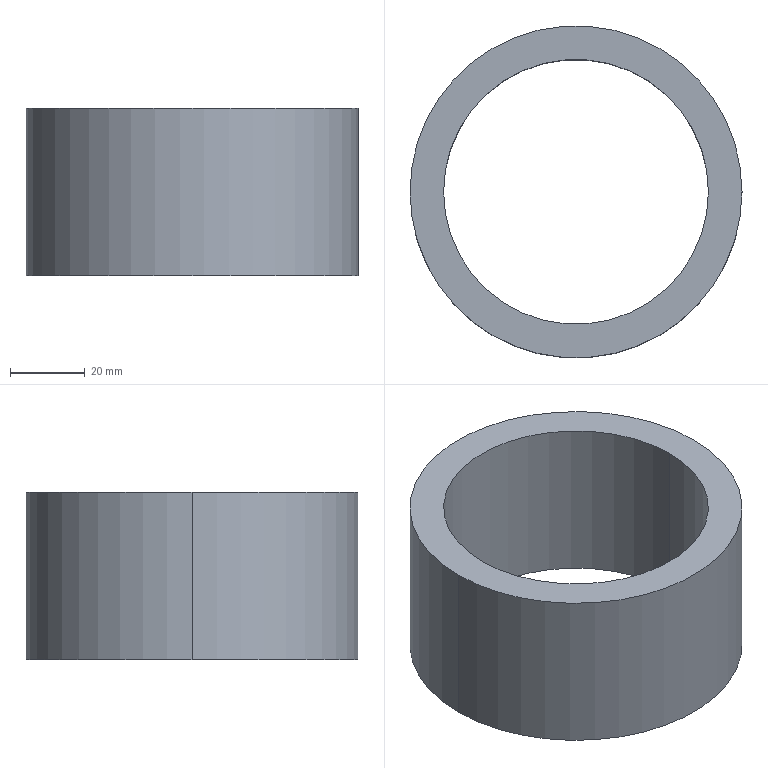Part | SolidWorks | features Extrusion 1 | 1 solid | 6 faces | box 89 x 89 x 45 mm | volume 101788 mm3 | cylinder 4 | plane 2 | commonest cylinder face diameters 71 x2 89 x2
STEP:
#1=CARTESIAN_POINT('',(-35.5,0.,45.));
#2=VERTEX_POINT('',#1);
#3=CARTESIAN_POINT('',(35.5,0.,45.));
#4=VERTEX_POINT('',#3);
#5=CARTESIAN_POINT('',(0.,0.,45.));
#6=DIRECTION('',(0.,0.,1.));
#7=DIRECTION('',(1.,0.,0.));
#8=AXIS2_PLACEMENT_3D('',#5,#6,#7);
#9=CIRCLE('',#8,35.5);
#10=EDGE_CURVE('',#2,#4,#9,.T.);
#11=ORIENTED_EDGE('',*,*,#10,.T.);
#12=CARTESIAN_POINT('',(35.5,0.,0.));
#13=VERTEX_POINT('',#12);
#14=CARTESIAN_POINT('',(35.5,0.,45.));
#15=DIRECTION('',(0.,0.,-1.));
#16=VECTOR('',#15,1000.);
#17=LINE('',#14,#16);
#18=EDGE_CURVE('',#4,#13,#17,.T.);
#19=ORIENTED_EDGE('',*,*,#18,.T.);
#20=CARTESIAN_POINT('',(-35.5,0.,0.));
#21=VERTEX_POINT('',#20);
#22=CARTESIAN_POINT('',(0.,0.,0.));
#23=DIRECTION('',(0.,0.,1.));
#24=DIRECTION('',(1.,0.,0.));
#25=AXIS2_PLACEMENT_3D('',#22,#23,#24);
#26=CIRCLE('',#25,35.5);
#27=EDGE_CURVE('',#21,#13,#26,.T.);
#28=ORIENTED_EDGE('',*,*,#27,.F.);
#29=CARTESIAN_POINT('',(-35.5,0.,45.));
#30=DIRECTION('',(0.,0.,-1.));
#31=VECTOR('',#30,1000.);
#32=LINE('',#29,#31);
#33=EDGE_CURVE('',#2,#21,#32,.T.);
#34=ORIENTED_EDGE('',*,*,#33,.F.);
#35=EDGE_LOOP('',(#11,#19,#28,#34));
#36=FACE_OUTER_BOUND('',#35,.T.);
#37=CARTESIAN_POINT('',(0.,0.,45.));
#38=DIRECTION('',(0.,0.,-1.));
#39=DIRECTION('',(-1.,0.,0.));
#40=AXIS2_PLACEMENT_3D('',#37,#38,#39);
#41=CYLINDRICAL_SURFACE('',#40,35.5);
#42=ADVANCED_FACE('',(#36),#41,.F.);
#43=CARTESIAN_POINT('',(44.5,0.,45.));
#44=VERTEX_POINT('',#43);
#45=CARTESIAN_POINT('',(-44.5,0.,45.));
#46=VERTEX_POINT('',#45);
#47=CARTESIAN_POINT('',(0.,0.,45.));
#48=DIRECTION('',(0.,0.,1.));
#49=DIRECTION('',(1.,0.,0.));
#50=AXIS2_PLACEMENT_3D('',#47,#48,#49);
#51=CIRCLE('',#50,44.5);
#52=EDGE_CURVE('',#44,#46,#51,.T.);
#53=ORIENTED_EDGE('',*,*,#52,.F.);
#54=CARTESIAN_POINT('',(44.5,0.,0.));
#55=VERTEX_POINT('',#54);
#56=CARTESIAN_POINT('',(44.5,0.,45.));
#57=DIRECTION('',(0.,0.,-1.));
#58=VECTOR('',#57,1000.);
#59=LINE('',#56,#58);
#60=EDGE_CURVE('',#44,#55,#59,.T.);
#61=ORIENTED_EDGE('',*,*,#60,.T.);
#62=CARTESIAN_POINT('',(-44.5,0.,0.));
#63=VERTEX_POINT('',#62);
#64=CARTESIAN_POINT('',(0.,0.,0.));
#65=DIRECTION('',(0.,0.,1.));
#66=DIRECTION('',(1.,0.,0.));
#67=AXIS2_PLACEMENT_3D('',#64,#65,#66);
#68=CIRCLE('',#67,44.5);
#69=EDGE_CURVE('',#55,#63,#68,.T.);
#70=ORIENTED_EDGE('',*,*,#69,.T.);
#71=CARTESIAN_POINT('',(-44.5,0.,45.));
#72=DIRECTION('',(0.,0.,-1.));
#73=VECTOR('',#72,1000.);
#74=LINE('',#71,#73);
#75=EDGE_CURVE('',#46,#63,#74,.T.);
#76=ORIENTED_EDGE('',*,*,#75,.F.);
#77=EDGE_LOOP('',(#53,#61,#70,#76));
#78=FACE_OUTER_BOUND('',#77,.T.);
#79=CARTESIAN_POINT('',(0.,0.,45.));
#80=DIRECTION('',(0.,0.,-1.));
#81=DIRECTION('',(-1.,0.,0.));
#82=AXIS2_PLACEMENT_3D('',#79,#80,#81);
#83=CYLINDRICAL_SURFACE('',#82,44.5);
#84=ADVANCED_FACE('',(#78),#83,.T.);
#85=CARTESIAN_POINT('',(0.,0.,45.));
#86=DIRECTION('',(0.,0.,1.));
#87=DIRECTION('',(1.,0.,0.));
#88=AXIS2_PLACEMENT_3D('',#85,#86,#87);
#89=CIRCLE('',#88,44.5);
#90=EDGE_CURVE('',#46,#44,#89,.T.);
#91=ORIENTED_EDGE('',*,*,#90,.T.);
#92=ORIENTED_EDGE('',*,*,#52,.T.);
#93=EDGE_LOOP('',(#91,#92));
#94=FACE_OUTER_BOUND('',#93,.T.);
#95=ORIENTED_EDGE('',*,*,#10,.F.);
#96=CARTESIAN_POINT('',(0.,0.,45.));
#97=DIRECTION('',(0.,0.,1.));
#98=DIRECTION('',(1.,0.,0.));
#99=AXIS2_PLACEMENT_3D('',#96,#97,#98);
#100=CIRCLE('',#99,35.5);
#101=EDGE_CURVE('',#4,#2,#100,.T.);
#102=ORIENTED_EDGE('',*,*,#101,.F.);
#103=EDGE_LOOP('',(#95,#102));
#104=FACE_BOUND('',#103,.T.);
#105=CARTESIAN_POINT('',(0.,0.,45.));
#106=DIRECTION('',(0.,0.,1.));
#107=DIRECTION('',(1.,0.,0.));
#108=AXIS2_PLACEMENT_3D('',#105,#106,#107);
#109=PLANE('',#108);
#110=ADVANCED_FACE('',(#94,#104),#109,.T.);
#111=CARTESIAN_POINT('',(0.,0.,0.));
#112=DIRECTION('',(0.,0.,1.));
#113=DIRECTION('',(1.,0.,0.));
#114=AXIS2_PLACEMENT_3D('',#111,#112,#113);
#115=CIRCLE('',#114,44.5);
#116=EDGE_CURVE('',#63,#55,#115,.T.);
#117=ORIENTED_EDGE('',*,*,#116,.F.);
#118=ORIENTED_EDGE('',*,*,#69,.F.);
#119=EDGE_LOOP('',(#117,#118));
#120=FACE_OUTER_BOUND('',#119,.T.);
#121=ORIENTED_EDGE('',*,*,#27,.T.);
#122=CARTESIAN_POINT('',(0.,0.,0.));
#123=DIRECTION('',(0.,0.,1.));
#124=DIRECTION('',(1.,0.,0.));
#125=AXIS2_PLACEMENT_3D('',#122,#123,#124);
#126=CIRCLE('',#125,35.5);
#127=EDGE_CURVE('',#13,#21,#126,.T.);
#128=ORIENTED_EDGE('',*,*,#127,.T.);
#129=EDGE_LOOP('',(#121,#128));
#130=FACE_BOUND('',#129,.T.);
#131=CARTESIAN_POINT('',(0.,0.,0.));
#132=DIRECTION('',(0.,0.,1.));
#133=DIRECTION('',(1.,0.,0.));
#134=AXIS2_PLACEMENT_3D('',#131,#132,#133);
#135=PLANE('',#134);
#136=ADVANCED_FACE('',(#120,#130),#135,.F.);
#137=ORIENTED_EDGE('',*,*,#60,.F.);
#138=ORIENTED_EDGE('',*,*,#90,.F.);
#139=ORIENTED_EDGE('',*,*,#75,.T.);
#140=ORIENTED_EDGE('',*,*,#116,.T.);
#141=EDGE_LOOP('',(#137,#138,#139,#140));
#142=FACE_OUTER_BOUND('',#141,.T.);
#143=CARTESIAN_POINT('',(0.,0.,45.));
#144=DIRECTION('',(0.,0.,-1.));
#145=DIRECTION('',(-1.,0.,0.));
#146=AXIS2_PLACEMENT_3D('',#143,#144,#145);
#147=CYLINDRICAL_SURFACE('',#146,44.5);
#148=ADVANCED_FACE('',(#142),#147,.T.);
#149=ORIENTED_EDGE('',*,*,#18,.F.);
#150=ORIENTED_EDGE('',*,*,#101,.T.);
#151=ORIENTED_EDGE('',*,*,#33,.T.);
#152=ORIENTED_EDGE('',*,*,#127,.F.);
#153=EDGE_LOOP('',(#149,#150,#151,#152));
#154=FACE_OUTER_BOUND('',#153,.T.);
#155=CARTESIAN_POINT('',(0.,0.,45.));
#156=DIRECTION('',(0.,0.,-1.));
#157=DIRECTION('',(-1.,0.,0.));
#158=AXIS2_PLACEMENT_3D('',#155,#156,#157);
#159=CYLINDRICAL_SURFACE('',#158,35.5);
#160=ADVANCED_FACE('',(#154),#159,.F.);
#161=CLOSED_SHELL('',(#42,#84,#110,#136,#148,#160));
#162=MANIFOLD_SOLID_BREP('',#161);
#163=CARTESIAN_POINT('',(0.,0.,0.));
#164=DIRECTION('',(0.,0.,1.));
#165=DIRECTION('',(1.,0.,0.));
#166=AXIS2_PLACEMENT_3D('',#163,#164,#165);
#167=(LENGTH_UNIT()NAMED_UNIT(*)SI_UNIT(.MILLI.,.METRE.));
#168=UNCERTAINTY_MEASURE_WITH_UNIT(LENGTH_MEASURE(0.00001),#167,'','');
#169=(NAMED_UNIT(*)PLANE_ANGLE_UNIT()SI_UNIT($,.RADIAN.));
#170=(NAMED_UNIT(*)SI_UNIT($,.STERADIAN.)SOLID_ANGLE_UNIT());
#171=(GEOMETRIC_REPRESENTATION_CONTEXT(3)GLOBAL_UNCERTAINTY_ASSIGNED_CONTEXT((#168))GLOBAL_UNIT_ASSIGNED_CONTEXT((#167,#169,#170))REPRESENTATION_CONTEXT('',''));
#172=ADVANCED_BREP_SHAPE_REPRESENTATION('',(#162,#166),#171);